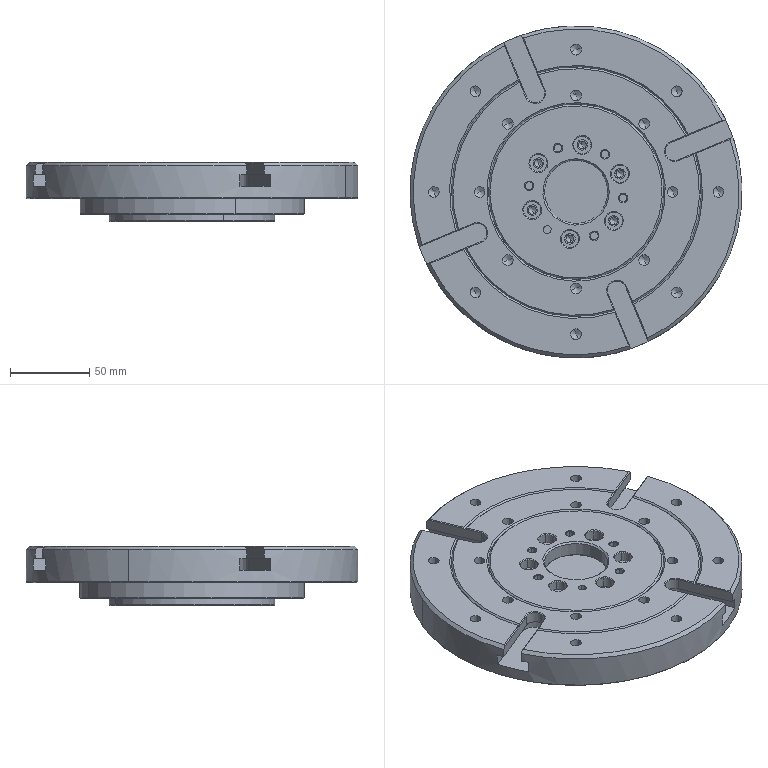NC program | Mastercam | posted with a generic post
Whole program:
%
:0001()
(MATERIAL - ALUMINUM MM - 2024)
(T10|50 INC |H10|XY STOCK TO LEAVE - 0.|Z STOCK TO LEAVE - .05)
(T4|12 FEMR |H4|XY STOCK TO LEAVE - .1|Z STOCK TO LEAVE - 0.)
(T2|8 CHM |H2)
(T3|3.5 DR |H3)
(T6|3 FEMR |H6|D6|WEAR COMP|TOOL DIA. - 3.|XY STOCK TO LEAVE - .03|Z STOCK TO LEAVE - 0.)
(T7|3 FEMF |H7|D7|WEAR COMP|TOOL DIA. - 3.|XY STOCK TO LEAVE - .02|Z STOCK TO LEAVE - 0.)
(T9|12 FEMF |H9|D9|WEAR COMP|TOOL DIA. - 12.)
(T5|6 CBCHM |H5|D5|WEAR COMP|TOOL DIA. - 6.|XY STOCK TO LEAVE - -.5|Z STOCK TO LEAVE - 0.)
(T8|26 60DGEA |H8|D8|WEAR COMP|TOOL DIA. - 26.)
(T1|2 FEMR |H1|D1|WEAR COMP|TOOL DIA. - 2.|XY STOCK TO LEAVE - .05|Z STOCK TO LEAVE - .05)
(T12|5.5 DR |H12)
(T13|5.5 FL |H13)
N100 G21
N102 G0 G17 G40 G80 G90 G94 G98
N104 G0 G28 G91 Z0.
N106 G0 G28 X0. Y0.
(50 INC |TOOL - 10|DIA. OFF. - 10|LEN. - 10|TOOL DIA. - 50.)
N108 T10 M6
N110 G0 G54 G90 X2.5 Y-45. C180. B-90. S1600 M3
N112 G43 H10 Z51.
N114 Z2.
N116 G1 Z.525 F2000.
N118 Y-15. F800.
N120 Y15.
N122 Y45.
N124 Z.05 F2000.
N126 Y15. F800.
N128 Y-15.
N130 Y-45.
N132 G0 Z51.
N134 Y-52.5
N136 Z50.7
N138 Z1.7
N140 G1 Z0. F2000.
N142 Y-15. F400.
N144 Y15.
N146 Y52.5
N148 G0 Z50.7
N150 M5
N152 G0 G28 G91 Z0.
N154 G28 C0. B0.
N156 M01
N158 G0 G17 G40 G80 G90 G94 G98
N160 G0 G28 G91 Z0.
(12 FEMR |TOOL - 4|DIA. OFF. - 4|LEN. - 4|TOOL DIA. - 12.)
N162 T4 M6
N164 G0 G54 G90 X-15.368 Y12.05 C180. B-90. S3000 M3
N166 G43 H4 Z51.
N168 Z3.
N170 G1 Z-7.75 F2000.
N172 X-14.091 Y12.542 Z-7.887
N174 G3 X-13.152 Y13.152 Z-8. I-.97 J2.519
N176 X-11.887 Y14.177 I-17.737 J23.191
N178 G2 X-4.841 Y17.798 I12.129 J-14.934
N180 X-.037 Y18.437 I4.804 J-17.75
N182 X18.352 Y.048 J-18.389
N184 X16.721 Y-7.524 I-18.389
N186 X.057 Y-18.28 I-16.664 J7.531
N188 X-18.23 Y.007 J18.287
N190 X-17.453 Y5.28 I18.287
N192 X-14.145 Y11.487 I17.094 J-5.126
N194 X-4.518 Y17.504 I14.409 J-12.344
N196 X-.041 Y18.069 I4.477 J-17.459
N198 X17.983 Y.045 J-18.024
N200 X16.969 Y-5.915 I-18.024
N202 G1 X16.545 Y-7.009
N204 X16.05 Y-8.073
N206 X15.487 Y-9.102
N208 X14.858 Y-10.092
N210 X14.165 Y-11.039
N212 X13.412 Y-11.939
N214 X12.601 Y-12.787
N216 X11.737 Y-13.58
N218 X10.823 Y-14.316
N220 X9.862 Y-14.989
N222 X8.86 Y-15.599
N224 X7.82 Y-16.141
N226 X6.746 Y-16.615
N228 X5.644 Y-17.017
N230 X4.518 Y-17.346
N232 X3.372 Y-17.6
N234 X2.213 Y-17.78
N236 X1.044 Y-17.882
N238 X-.129 Y-17.909
N240 X-1.301 Y-17.858
N242 X-2.467 Y-17.731
N244 X-3.623 Y-17.527
N246 X-4.763 Y-17.249
N248 X-5.882 Y-16.897
N250 X-6.975 Y-16.472
N252 X-8.039 Y-15.976
N254 X-9.067 Y-15.412
N256 X-10.057 Y-14.782
N258 X-11.003 Y-14.088
N260 X-11.902 Y-13.334
N262 X-12.75 Y-12.523
N264 X-13.542 Y-11.658
N266 X-14.277 Y-10.743
N268 X-14.949 Y-9.782
N270 X-15.558 Y-8.778
N272 X-16.1 Y-7.738
N274 X-16.572 Y-6.664
N276 X-16.973 Y-5.561
N278 X-17.301 Y-4.435
N280 X-17.554 Y-3.289
N282 X-17.733 Y-2.129
N284 X-17.834 Y-.961
N286 X-17.859 Y.212
N288 X-17.808 Y1.384
N290 X-17.679 Y2.551
N292 X-17.475 Y3.706
N294 X-17.194 Y4.845
N296 G2 X-11.394 Y13.64 I16.405 J-4.509
N298 X-.054 Y17.688 I11.34 J-13.86
N300 X3.235 Y17.384 J-17.908
N302 X17.612 Y.06 I-3.249 J-17.324
N304 X11.732 Y-13.082 I-17.626
N306 X.051 Y-17.539 I-11.681 J13.078
N308 X-17.484 Y-.004 J17.535
N310 X-15.678 Y7.745 I17.535
N312 X-9.712 Y14.411 I15.494 J-7.865
N314 X-.082 Y17.317 I9.63 J-14.502
N316 X8.957 Y14.786 J-17.408
N318 X17.235 Y.061 I-8.957 J-14.725
N320 X6.644 Y-15.841 I-17.235
N322 X.049 Y-17.159 I-6.595 J15.835
N324 X-17.104 Y-.006 J17.153
N326 X-15.643 Y6.923 I17.153
N328 X-7.939 Y15.014 I15.49 J-7.034
N330 X-.086 Y16.938 I7.853 J-15.068
N332 X12.403 Y11.468 J-16.992
N334 X16.856 Y.06 I-12.385 J-11.408
N336 G1 X16.819 Y-1.057
N338 X16.708 Y-2.169
N340 X16.524 Y-3.271
N342 X16.266 Y-4.359
N344 X15.937 Y-5.427
N346 X15.538 Y-6.47
N348 X15.071 Y-7.486
N350 X14.537 Y-8.467
N352 X13.94 Y-9.412
N354 X13.281 Y-10.314
N356 X12.564 Y-11.171
N358 X11.791 Y-11.979
N360 X10.966 Y-12.733
N362 X10.094 Y-13.431
N364 X9.177 Y-14.07
N366 X8.219 Y-14.646
N368 X7.226 Y-15.158
N370 X6.2 Y-15.602
N372 X5.148 Y-15.978
N374 X4.073 Y-16.283
N376 X2.98 Y-16.516
N378 X1.874 Y-16.676
N380 G2 X.047 Y-16.777 I-1.827 J16.671
N382 X-16.724 Y-.006 J16.771
N384 X-15.795 Y5.496 I16.771
N386 X-7.624 Y14.747 I15.663 J-5.6
N388 X-.089 Y16.555 I7.535 J-14.797
N390 X12.695 Y10.547 J-16.605
N392 X16.472 Y.059 I-12.675 J-10.488
N394 X1.467 Y-16.328 I-16.452
N396 X.047 Y-16.39 I-1.42 J16.321
N398 X-16.336 Y-.007 J16.383
N400 X-15.681 Y4.579 I16.383
N402 X-6.765 Y14.729 I15.551 J-4.669
N404 X-.09 Y16.168 I6.675 J-14.767
N406 X13.306 Y9.08 J-16.206
N408 X16.081 Y.058 I-13.281 J-9.022
N410 X.43 Y-15.993 I-16.056
N412 X.045 Y-15.998 I-.385 J15.984
N414 X-15.944 Y-.009 J15.989
N416 X-15.511 Y3.683 I15.989
N418 X-5.813 Y14.701 I15.389 J-3.768
N420 X-.086 Y15.776 I5.727 J-14.713
N422 X14.101 Y6.914 J-15.788
N424 X15.685 Y.054 I-14.067 J-6.86
N426 X.034 Y-15.597 I-15.651
N428 X-1.89 Y-15.478 J15.651
N430 X-15.544 Y-.017 I1.927 J15.461
N432 X-15.155 Y3.441 I15.581
N434 X-3.002 Y15.094 I15.044 J-3.527
N436 X-.075 Y15.376 I2.927 J-15.075
N438 X15.21 Y1.502 J-15.357
N440 X15.281 Y.037 I-15.157 J-1.465
N442 X.053 Y-15.191 I-15.228
N444 X-7.895 Y-12.951 J15.228
N446 X-15.135 Y-.031 I7.908 J12.92
N448 X-14.566 Y4.081 I15.148
N450 X-.107 Y14.962 I14.459 J-4.166
N452 X10.238 Y10.842 J-15.047
N454 X14.868 Y.065 I-10.227 J-10.777
N456 X4.351 Y-14.144 I-14.857
N458 X.048 Y-14.785 I-4.303 J14.13
N460 X-14.723 Y-.014 J14.771
N462 X-14.544 Y2.276 I14.771
N464 X-.104 Y14.547 I14.44 J-2.361
N466 X9.642 Y10.827 J-14.632
N468 X14.452 Y.068 I-9.629 J-10.759
N470 X3.33 Y-13.985 I-14.439
N472 X.036 Y-14.367 I-3.294 J14.017
N474 X-13.878 Y-3.675 J14.399
N476 X-14.355 Y-.006 I13.878 J3.669
N478 X0. Y14.349 I14.355
N480 X9.197 Y11.015 J-14.355
N482 X14.35 Y0. I-9.197 J-11.015
N484 X0. Y-14.35 I-14.35
N486 X-4.701 Y-13.558 J14.35
N488 X-14.35 Y0. I4.701 J13.558
N490 X-11.861 Y8.077 I14.35
N492 G3 X-11.437 Y9.113 Z-7.884 I-2.232 J1.519
N494 G1 X-11.205 Y10.388 Z-7.75
N496 G0 Z51.
N498 M5
N500 G0 G28 G91 Z0.
N502 G28 C0. B0.
N504 M01
N506 G0 G17 G40 G80 G90 G94 G98
N508 G0 G28 G91 Z0.
(8 CHM |TOOL - 2|DIA. OFF. - 2|LEN. - 2|TOOL DIA. - 8.)
N510 T2 M6
N512 G0 G54 G90 X-3.35 Y-3.35 C180. B-90. S2000 M3
N514 G43 H2 Z100.
N516 G81 G98 Z-1. R1. F100.
N518 X3.35
N520 X0. Y0.
N522 X3.35 Y3.35
N524 G80
N526 Z125.
N528 Y-3.35
N530 B-270.
N532 G81 G98 Z23. R26. F100.
N534 X-3.35
N536 Y3.35
N538 G80
N540 M5
N542 G0 G28 G91 Z0.
N544 G28 C0. B0.
N546 M01
N548 G0 G17 G40 G80 G90 G94 G98
N550 G0 G28 G91 Z0.
(3.5 DR |TOOL - 3|DIA. OFF. - 3|LEN. - 3|TOOL DIA. - 3.5)
N552 T3 M6
N554 G0 G54 G90 X-3.35 Y-3.35 C180. B-90. S2000 M3
N556 G43 H3 Z50.
N558 G83 G98 Z-5. R1. Q2. F60.
N560 X3.35
N562 Y3.35
N564 G80
N566 X0. Y0.
N568 G83 G98 Z-7. R1. Q2. F100.
N570 G80
N572 M5
N574 G0 G28 G91 Z0.
N576 G28 C0. B0.
N578 M01
N580 G0 G17 G40 G80 G90 G94 G98
N582 G0 G28 G91 Z0.
(8 CHM |TOOL - 2|DIA. OFF. - 2|LEN. - 2|TOOL DIA. - 8.)
N584 T2 M6
N586 G0 G54 G90 X-3.35 Y-3.35 C180. B-90. S2000 M3
N588 G43 H2 Z50.
N590 G81 G98 Z-2.2 R1. F100.
N592 X3.35
N594 X0. Y0. Z-2.8
N596 X3.35 Y3.35 Z-2.2
N598 G80
N600 M5
N602 G0 G28 G91 Z0.
N604 G28 C0. B0.
N606 M01
N608 G0 G17 G40 G80 G90 G94 G98
N610 G0 G28 G91 Z0.
(3 FEMR |TOOL - 6|DIA. OFF. - 6|LEN. - 6|TOOL DIA. - 3.)
N612 T6 M6
N614 G0 G54 G90 X0. Y0. C180. B-90. S3500 M3
N616 G43 H6 Z46.8
N618 Z-1.2
N620 G1 Z-3.2 F2000.
N622 G41 D6 Y-.301 F300.
N624 G3 X.055 Y-.311 I.055 J.151
N626 X.109 Y-.301 J.161
N628 X.32 Y0. I-.109 J.301
N630 X0. Y.32 I-.32
N632 X-.32 Y0. J-.32
N634 X0. Y-.32 I.32
N636 X.109 Y-.301 J.32
N638 X.187 Y-.26 I-.109 J.301
N640 X.249 Y-.169 I-.094 J.13
N642 G1 G40 X0. Y0.
N644 G41 D6 Y-.442
N646 G3 X.08 Y-.456 I.08 J.221
N648 X.161 Y-.442 J.235
N650 X.47 Y0. I-.161 J.442
N652 X0. Y.47 I-.47
N654 X-.47 Y0. J-.47
N656 X0. Y-.47 I.47
N658 X.161 Y-.442 J.47
N660 X.266 Y-.387 I-.161 J.442
N662 X.36 Y-.256 I-.133 J.193
N664 G1 G40 X0. Y0.
N666 G0 Z46.8
N668 M5
N670 G0 G28 G91 Z0.
N672 G28 C0. B0.
N674 M01
N676 G0 G17 G40 G80 G90 G94 G98
N678 G0 G28 G91 Z0.
(3 FEMF |TOOL - 7|DIA. OFF. - 7|LEN. - 7|TOOL DIA. - 3.)
N680 T7 M6
N682 G0 G54 G90 X0. Y0. C180. B-90. S3500 M3
N684 G43 H7 Z46.8
N686 Z-1.2
N688 G1 Z-3.2 F2000.
N690 G41 D7 Y-.451 F200.
N692 G3 X.082 Y-.465 I.082 J.225
N694 X.164 Y-.451 J.239
N696 X.48 Y0. I-.164 J.451
N698 X0. Y.48 I-.48
N700 X-.48 Y0. J-.48
N702 X0. Y-.48 I.48
N704 X.164 Y-.451 J.48
N706 X.272 Y-.396 I-.164 J.451
N708 X.367 Y-.262 I-.136 J.198
N710 G1 G40 X0. Y0.
N712 G41 D7 Y-.451
N714 G3 X.082 Y-.465 I.082 J.225
N716 X.164 Y-.451 J.239
N718 X.48 Y0. I-.164 J.451
N720 X0. Y.48 I-.48
N722 X-.48 Y0. J-.48
N724 X0. Y-.48 I.48
N726 X.164 Y-.451 J.48
N728 X.272 Y-.396 I-.164 J.451
N730 X.367 Y-.262 I-.136 J.198
N732 G1 G40 X0. Y0.
N734 G41 D7 Y-.451
N736 G3 X.082 Y-.465 I.082 J.225
N738 X.164 Y-.451 J.239
N740 X.48 Y0. I-.164 J.451
N742 X0. Y.48 I-.48
N744 X-.48 Y0. J-.48
N746 X0. Y-.48 I.48
N748 X.164 Y-.451 J.48
N750 X.272 Y-.396 I-.164 J.451
N752 X.367 Y-.262 I-.136 J.198
N754 G1 G40 X0. Y0.
N756 G0 Z46.8
N758 M5
N760 G0 G28 G91 Z0.
N762 G28 C0. B0.
N764 M01
N766 G0 G17 G40 G80 G90 G94 G98
N768 G0 G28 G91 Z0.
(12 FEMF |TOOL - 9|DIA. OFF. - 9|LEN. - 9|TOOL DIA. - 12.)
N770 T9 M6
N772 G0 G54 G90 X.864 Y17.736 C180. B-90. S3500 M3
N774 G43 H9 Z50.7
N776 Z1.7
N778 G1 Z-8. F2000.
N780 G41 D9 X.634 Y14.745 F600.
N782 G3 X.632 Y14.706 I.499 J-.039
N784 X1.094 Y14.208 I.501
N786 G2 X14.25 Y0. I-1.094 J-14.208
N788 X0. Y-14.25 I-14.25
N790 X-14.25 Y0. J14.25
N792 X0. Y14.25 I14.25
N794 X1.094 Y14.208 J-14.25
N796 X1.592 Y14.161 I-1.094 J-14.208
N798 G3 X1.648 Y14.158 I.056 J.497
N800 X2.145 Y14.602 J.5
N802 G1 G40 X2.48 Y17.583
N804 G0 Z50.7
N806 M5
N808 G0 G28 G91 Z0.
N810 G28 C0. B0.
N812 M01
N814 G0 G17 G40 G80 G90 G94 G98
N816 G0 G28 G91 Z0.
(6 CBCHM |TOOL - 5|DIA. OFF. - 5|LEN. - 5|TOOL DIA. - 6.)
N818 T5 M6
N820 G0 G54 G90 X-.166 Y12.259 C180. B-90. S3500 M3
N822 G43 H5 Z50.
N824 Z1.
N826 G1 Z-1.5 F2000.
N828 G41 D5 X-.247 Y9.26 F600.
N830 Y9.247
N832 G3 X.239 Y8.747 I.499
N834 G2 X8.75 Y0. I-.239 J-8.747
N836 X0. Y-8.75 I-8.75
N838 X-8.75 Y0. J8.75
N840 X0. Y8.75 I8.75
N842 X.239 Y8.747 J-8.75
N844 X.738 Y8.719 I-.239 J-8.747
N846 G3 X.78 Y8.717 I.042 J.498
N848 X1.278 Y9.175 J.5
N850 G1 G40 X1.531 Y12.164
N852 G0 Z50.
N854 M5
N856 G0 G28 G91 Z0.
N858 G28 C0. B0.
N860 M01
N862 G0 G17 G40 G80 G90 G94 G98
N864 G0 G28 G91 Z0.
(26 60DGEA |TOOL - 8|DIA. OFF. - 8|LEN. - 8|TOOL DIA. - 26.)
N866 T8 M6
N868 G0 G54 G90 X4.66 Y-15.4 C0. B0. S4000 M3
N870 G43 H8 Z50.
N872 Z7.875
N874 G1 Z1.675 F2000.
N876 G41 D8 Y-12.4 F1000.
N878 G3 X4.56 Y-12.3 I-.1
N880 G1 X-4.56
N882 G3 X-4.66 Y-12.4 J-.1
N884 G1 G40 Y-15.4
N886 G0 Z16.875
N888 X6.135
N890 Z6.625
N892 G1 Z.425 F2000.
N894 G41 D8 Y-12.4 F1000.
N896 G3 X6.035 Y-12.3 I-.1
N898 G1 X-6.035
N900 G3 X-6.135 Y-12.4 J-.1
N902 G1 G40 Y-15.4
N904 G0 Z15.625
N906 X7.094
N908 Z5.375
N910 G1 Z-.825 F2000.
N912 G41 D8 Y-12.4 F1000.
N914 G3 X6.994 Y-12.3 I-.1
N916 G1 X-6.994
N918 G3 X-7.094 Y-12.4 J-.1
N920 G1 G40 Y-15.4
N922 G0 Z14.375
N924 X7.735
N926 Z4.125
N928 G1 Z-2.075 F2000.
N930 G41 D8 Y-12.4 F1000.
N932 G3 X7.635 Y-12.3 I-.1
N934 G1 X-7.635
N936 G3 X-7.735 Y-12.4 J-.1
N938 G1 G40 Y-15.4
N940 G0 Z13.125
N942 X8.134
N944 Z2.875
N946 G1 Z-3.325 F2000.
N948 G41 D8 Y-12.4 F1000.
N950 G3 X8.034 Y-12.3 I-.1
N952 G1 X-8.034
N954 G3 X-8.134 Y-12.4 J-.1
N956 G1 G40 Y-15.4
N958 G0 Z11.875
N960 X8.418
N962 Z1.625
N964 G1 Z-4.575 F2000.
N966 G41 D8 Y-12.4 F1000.
N968 G3 X8.318 Y-12.3 I-.1
N970 G1 X-8.318
N972 G3 X-8.418 Y-12.4 J-.1
N974 G1 G40 Y-15.4
N976 G0 Z10.625
N978 X8.418
N980 Z.375
N982 G1 Z-5.825 F2000.
N984 G41 D8 Y-12.4 F1000.
N986 G3 X8.318 Y-12.3 I-.1
N988 G1 X-8.318
N990 G3 X-8.418 Y-12.4 J-.1
N992 G1 G40 Y-15.4
N994 G0 Z9.375
N996 X8.134
N998 Z-.875
N1000 G1 Z-7.075 F2000.
N1002 G41 D8 Y-12.4 F1000.
N1004 G3 X8.034 Y-12.3 I-.1
N1006 G1 X-8.034
N1008 G3 X-8.134 Y-12.4 J-.1
N1010 G1 G40 Y-15.4
N1012 G0 Z8.125
N1014 X7.735
N1016 Z-2.125
N1018 G1 Z-8.325 F2000.
N1020 G41 D8 Y-12.4 F1000.
N1022 G3 X7.635 Y-12.3 I-.1
N1024 G1 X-7.635
N1026 G3 X-7.735 Y-12.4 J-.1
N1028 G1 G40 Y-15.4
N1030 G0 Z6.875
N1032 X7.094
N1034 Z-3.375
N1036 G1 Z-9.575 F2000.
N1038 G41 D8 Y-12.4 F1000.
N1040 G3 X6.994 Y-12.3 I-.1
N1042 G1 X-7.433
N1044 G3 X-7.533 Y-12.4 J-.1
N1046 G1 G40 Y-15.4
N1048 G0 Z5.625
N1050 X6.518
N1052 Z-4.625
N1054 G1 Z-10.825 F2000.
N1056 G41 D8 Y-12.4 F1000.
N1058 G3 X6.418 Y-12.3 I-.1
N1060 G1 X-6.079
N1062 G3 X-6.179 Y-12.4 J-.1
N1064 G1 G40 Y-15.4
N1066 G0 Z4.375
N1068 X4.413
N1070 Z-5.875
N1072 G1 Z-12.075 F2000.
N1074 G41 D8 Y-12.4 F1000.
N1076 G3 X4.313 Y-12.3 I-.1
N1078 G1 X-3.974
N1080 G3 X-4.074 Y-12.4 J-.1
N1082 G1 G40 Y-15.4
N1084 G0 Z50.
N1086 M5
N1088 G0 G28 G91 Z0.
N1090 G28
N1092 M01
N1094 G0 G17 G40 G80 G90 G94 G98
N1096 G0 G28 G91 Z0.
(2 FEMR |TOOL - 1|DIA. OFF. - 1|LEN. - 1|TOOL DIA. - 2.)
N1098 T1 M6
N1100 G0 G54 G90 X.55 Y-.132 C-108.997 B-90. S4500 M3
N1102 G43 H1 Z107.627
N1104 Z8.627
N1106 G1 Z7.483 F2000.
N1108 G41 D1 Y1.868 F600.
N1110 Y8.741
N1112 X-.55
N1114 Y1.868
N1116 G40 Y-.132
N1118 X.55
N1120 Z7.34 F2000.
N1122 G41 D1 Y1.868 F600.
N1124 Y8.741
N1126 X-.55
N1128 Y1.868
N1130 G40 Y-.132
N1132 X.55
N1134 Z7.197 F2000.
N1136 G41 D1 Y1.868 F600.
N1138 Y8.741
N1140 X-.55
N1142 Y1.868
N1144 G40 Y-.132
N1146 X.55
N1148 Z7.053 F2000.
N1150 G41 D1 Y1.868 F600.
N1152 Y8.741
N1154 X-.55
N1156 Y1.868
N1158 G40 Y-.132
N1160 X.55
N1162 Z6.91 F2000.
N1164 G41 D1 Y1.868 F600.
N1166 Y8.741
N1168 X-.55
N1170 Y1.868
N1172 G40 Y-.132
N1174 X.55
N1176 Z6.767 F2000.
N1178 G41 D1 Y1.868 F600.
N1180 Y8.741
N1182 X-.55
N1184 Y1.868
N1186 G40 Y-.132
N1188 X.55
N1190 Z6.623 F2000.
N1192 G41 D1 Y1.868 F600.
N1194 Y8.741
N1196 X-.55
N1198 Y1.868
N1200 G40 Y-.132
N1202 X.55
N1204 Z6.48 F2000.
N1206 G41 D1 Y1.868 F600.
N1208 Y8.741
N1210 X-.55
N1212 Y1.868
N1214 G40 Y-.132
N1216 X.55
N1218 Z6.337 F2000.
N1220 G41 D1 Y1.868 F600.
N1222 Y8.741
N1224 X-.55
N1226 Y1.868
N1228 G40 Y-.132
N1230 X.55
N1232 Z6.193 F2000.
N1234 G41 D1 Y1.868 F600.
N1236 Y8.741
N1238 X-.55
N1240 Y1.868
N1242 G40 Y-.132
N1244 X.55
N1246 Z6.05 F2000.
N1248 G41 D1 Y1.868 F600.
N1250 Y8.741
N1252 X-.55
N1254 Y1.868
N1256 G40 Y-.132
N1258 X.55
N1260 Z5.907 F2000.
N1262 G41 D1 Y1.868 F600.
N1264 Y8.741
N1266 X-.55
N1268 Y1.868
N1270 G40 Y-.132
N1272 X.55
N1274 Z5.763 F2000.
N1276 G41 D1 Y1.868 F600.
N1278 Y8.741
N1280 X-.55
N1282 Y1.868
N1284 G40 Y-.132
N1286 X.55
N1288 Z5.62 F2000.
N1290 G41 D1 Y1.868 F600.
N1292 Y8.741
N1294 X-.55
N1296 Y1.868
N1298 G40 Y-.132
N1300 X.55
N1302 Z5.477 F2000.
N1304 G41 D1 Y1.868 F600.
N1306 Y8.741
N1308 X-.55
N1310 Y1.868
N1312 G40 Y-.132
N1314 G0 Z107.627
N1316 X.6
N1318 Z8.627
N1320 G1 Z5.427 F2000.
N1322 G41 D1 Y1.868 F600.
N1324 Y8.791
N1326 X-.6
N1328 Y1.868
N1330 G40 Y-.132
N1332 G0 Z107.627
N1334 C-71.003 B-270.
N1336 X.55
N1338 Z8.627
N1340 G1 Z7.483 F2000.
N1342 G41 D1 Y1.868 F600.
N1344 Y8.741
N1346 X-.55
N1348 Y1.868
N1350 G40 Y-.132
N1352 X.55
N1354 Z7.34 F2000.
N1356 G41 D1 Y1.868 F600.
N1358 Y8.741
N1360 X-.55
N1362 Y1.868
N1364 G40 Y-.132
N1366 X.55
N1368 Z7.197 F2000.
N1370 G41 D1 Y1.868 F600.
N1372 Y8.741
N1374 X-.55
N1376 Y1.868
N1378 G40 Y-.132
N1380 X.55
N1382 Z7.053 F2000.
N1384 G41 D1 Y1.868 F600.
N1386 Y8.741
N1388 X-.55
N1390 Y1.868
N1392 G40 Y-.132
N1394 X.55
N1396 Z6.91 F2000.
N1398 G41 D1 Y1.868 F600.
N1400 Y8.741
N1402 X-.55
N1404 Y1.868
N1406 G40 Y-.132
N1408 X.55
N1410 Z6.767 F2000.
N1412 G41 D1 Y1.868 F600.
N1414 Y8.741
N1416 X-.55
N1418 Y1.868
N1420 G40 Y-.132
N1422 X.55
N1424 Z6.623 F2000.
N1426 G41 D1 Y1.868 F600.
N1428 Y8.741
N1430 X-.55
N1432 Y1.868
N1434 G40 Y-.132
N1436 X.55
N1438 Z6.48 F2000.
N1440 G41 D1 Y1.868 F600.
N1442 Y8.741
N1444 X-.55
N1446 Y1.868
N1448 G40 Y-.132
N1450 X.55
N1452 Z6.337 F2000.
N1454 G41 D1 Y1.868 F600.
N1456 Y8.741
N1458 X-.55
N1460 Y1.868
N1462 G40 Y-.132
N1464 X.55
N1466 Z6.193 F2000.
N1468 G41 D1 Y1.868 F600.
N1470 Y8.741
N1472 X-.55
N1474 Y1.868
N1476 G40 Y-.132
N1478 X.55
N1480 Z6.05 F2000.
N1482 G41 D1 Y1.868 F600.
N1484 Y8.741
N1486 X-.55
N1488 Y1.868
N1490 G40 Y-.132
N1492 X.55
N1494 Z5.907 F2000.
N1496 G41 D1 Y1.868 F600.
N1498 Y8.741
N1500 X-.55
N1502 Y1.868
N1504 G40 Y-.132
N1506 X.55
N1508 Z5.763 F2000.
N1510 G41 D1 Y1.868 F600.
N1512 Y8.741
N1514 X-.55
N1516 Y1.868
N1518 G40 Y-.132
N1520 X.55
N1522 Z5.62 F2000.
N1524 G41 D1 Y1.868 F600.
N1526 Y8.741
N1528 X-.55
N1530 Y1.868
N1532 G40 Y-.132
N1534 X.55
N1536 Z5.477 F2000.
N1538 G41 D1 Y1.868 F600.
N1540 Y8.741
N1542 X-.55
N1544 Y1.868
N1546 G40 Y-.132
N1548 G0 Z107.627
N1550 X.6
N1552 Z8.627
N1554 G1 Z5.427 F2000.
N1556 G41 D1 Y1.868 F600.
N1558 Y8.791
N1560 X-.6
N1562 Y1.868
N1564 G40 Y-.132
N1566 G0 Z107.627
N1568 M5
N1570 G0 G28 G91 Z0.
N1572 G28 C0. B0.
N1574 M01
N1576 G0 G17 G40 G80 G90 G94 G98
N1578 G0 G28 G91 Z0.
(5.5 DR |TOOL - 12|DIA. OFF. - 12|LEN. - 12|TOOL DIA. - 5.5)
N1580 T12 M6
N1582 G0 G54 G90 X3.35 Y-3.35 C0. B-90. S2000 M3
N1584 G43 H12 Z75.
N1586 G83 G98 Z3. R26. Q2. F80.
N1588 Y3.35
N1590 X-3.35
N1592 G80
N1594 M5
N1596 G0 G28 G91 Z0.
N1598 G28 B0.
N1600 M01
N1602 G0 G17 G40 G80 G90 G94 G98
N1604 G0 G28 G91 Z0.
(5.5 FL |TOOL - 13|DIA. OFF. - 13|LEN. - 13|TOOL DIA. - 5.5)
N1606 T13 M6
N1608 G0 G54 G90 X3.35 Y-3.35 C0. B-90. S1000 M3
N1610 G43 H13 Z56.
N1612 G81 G98 Z3.5 R7. F80.
N1614 Y3.35
N1616 X-3.35
N1618 G80
N1620 M5
N1622 G0 G28 G91 Z0.
N1624 G0 G28 X0. Y0.
N1626 G28 B0.
N1628 M30
%